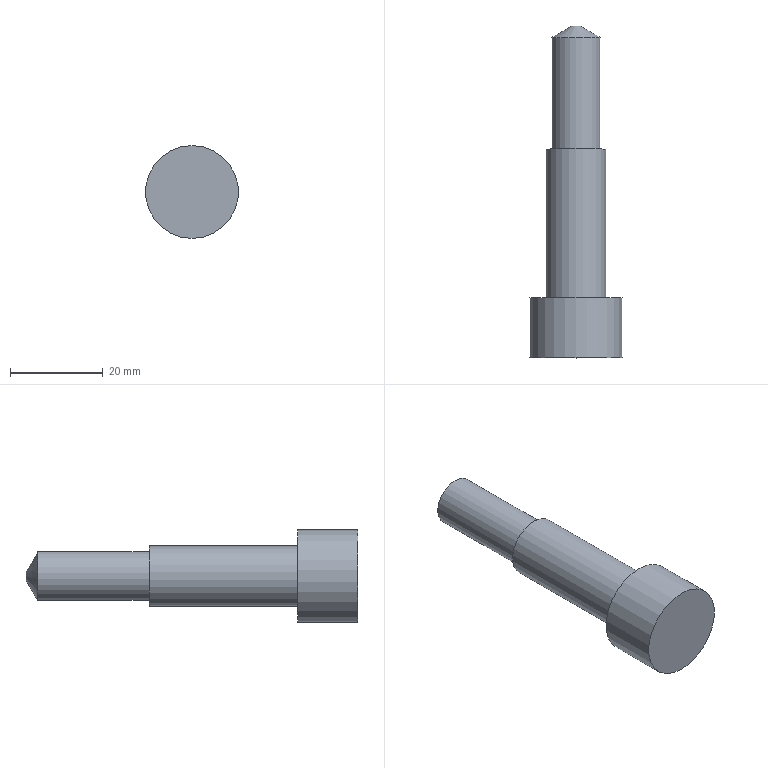Part | STEP file | solid 165 | 1 solid | 8 faces | box 20 x 71.5 x 20 mm | volume 10497 mm3 | plane 4 | cylinder 3 | cone 1 | commonest cylinder face diameters 10.5 x1 13 x1 20 x1